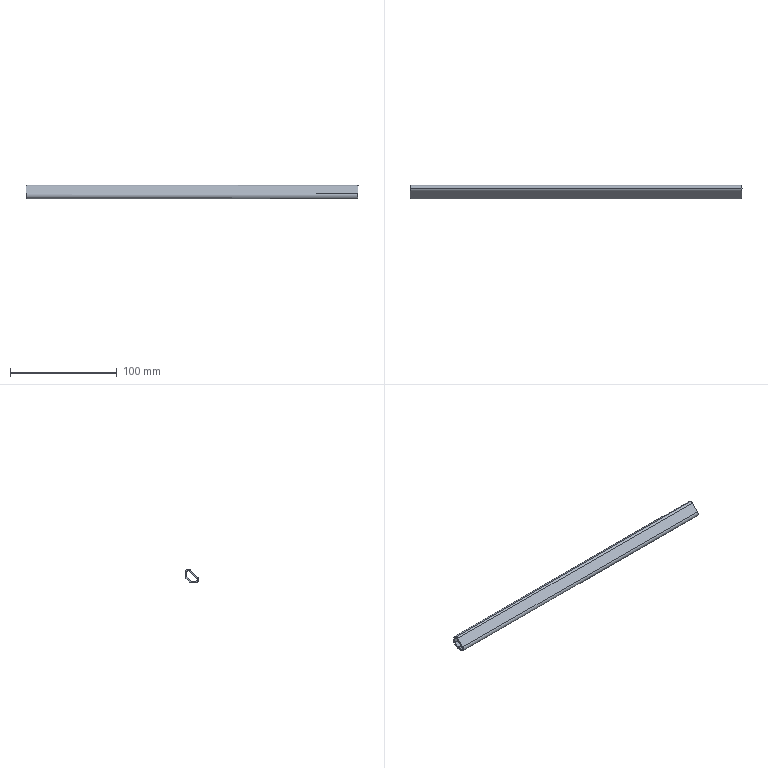Part | SolidWorks | features BaseBody 1 | 1 solid | 20 faces | box 311.635 x 12.741 x 12.993 mm | volume 16541 mm3 | cylinder 10 | plane 10 | commonest cylinder face diameters 3 x3 6 x3 1 x2 4 x2
STEP:
#1=CARTESIAN_POINT('',(151.49,213.806,-273.62));
#2=VERTEX_POINT('',#1);
#3=CARTESIAN_POINT('',(151.488,216.807,-276.619));
#4=VERTEX_POINT('',#3);
#5=CARTESIAN_POINT('',(151.488,213.807,-276.62));
#6=DIRECTION('',(-1.,-0.00003863,0.0008339));
#7=DIRECTION('',(0.0008339,-0.0004454,1.));
#8=AXIS2_PLACEMENT_3D('',#5,#6,#7);
#9=CIRCLE('',#8,3.);
#10=EDGE_CURVE('',#2,#4,#9,.T.);
#11=ORIENTED_EDGE('',*,*,#10,.T.);
#12=CARTESIAN_POINT('',(-160.136,216.795,-276.359));
#13=VERTEX_POINT('',#12);
#14=CARTESIAN_POINT('',(-160.136,216.795,-276.359));
#15=DIRECTION('',(1.,0.00003863,-0.0008339));
#16=VECTOR('',#15,1000.);
#17=LINE('',#14,#16);
#18=EDGE_CURVE('',#13,#4,#17,.T.);
#19=ORIENTED_EDGE('',*,*,#18,.F.);
#20=CARTESIAN_POINT('',(-160.134,213.794,-273.36));
#21=VERTEX_POINT('',#20);
#22=CARTESIAN_POINT('',(-160.136,213.795,-276.36));
#23=DIRECTION('',(1.,0.00003863,-0.0008339));
#24=DIRECTION('',(-0.00003826,1.,0.0004455));
#25=AXIS2_PLACEMENT_3D('',#22,#23,#24);
#26=CIRCLE('',#25,3.);
#27=EDGE_CURVE('',#13,#21,#26,.T.);
#28=ORIENTED_EDGE('',*,*,#27,.T.);
#29=CARTESIAN_POINT('',(-160.134,213.794,-273.36));
#30=DIRECTION('',(1.,0.00003863,-0.0008339));
#31=VECTOR('',#30,1000.);
#32=LINE('',#29,#31);
#33=EDGE_CURVE('',#21,#2,#32,.T.);
#34=ORIENTED_EDGE('',*,*,#33,.T.);
#35=EDGE_LOOP('',(#11,#19,#28,#34));
#36=FACE_OUTER_BOUND('',#35,.T.);
#37=CARTESIAN_POINT('',(48.652,213.803,-276.535));
#38=DIRECTION('',(-1.,-0.00003863,0.0008339));
#39=DIRECTION('',(0.0008339,-0.0004454,1.));
#40=AXIS2_PLACEMENT_3D('',#37,#38,#39);
#41=CYLINDRICAL_SURFACE('',#40,3.);
#42=ADVANCED_FACE('',(#36),#41,.T.);
#43=ORIENTED_EDGE('',*,*,#33,.F.);
#44=CARTESIAN_POINT('',(-160.134,211.673,-274.24));
#45=VERTEX_POINT('',#44);
#46=CARTESIAN_POINT('',(-160.136,213.795,-276.36));
#47=DIRECTION('',(1.,0.00003863,-0.0008339));
#48=DIRECTION('',(0.0008339,-0.0004454,1.));
#49=AXIS2_PLACEMENT_3D('',#46,#47,#48);
#50=CIRCLE('',#49,3.);
#51=EDGE_CURVE('',#21,#45,#50,.T.);
#52=ORIENTED_EDGE('',*,*,#51,.T.);
#53=CARTESIAN_POINT('',(151.49,211.685,-274.5));
#54=VERTEX_POINT('',#53);
#55=CARTESIAN_POINT('',(-160.134,211.673,-274.24));
#56=DIRECTION('',(1.,0.00003863,-0.0008339));
#57=VECTOR('',#56,1000.);
#58=LINE('',#55,#57);
#59=EDGE_CURVE('',#45,#54,#58,.T.);
#60=ORIENTED_EDGE('',*,*,#59,.T.);
#61=CARTESIAN_POINT('',(151.488,213.807,-276.62));
#62=DIRECTION('',(-1.,-0.00003863,0.0008339));
#63=DIRECTION('',(0.0006167,-0.7074,0.7068));
#64=AXIS2_PLACEMENT_3D('',#61,#62,#63);
#65=CIRCLE('',#64,3.);
#66=EDGE_CURVE('',#54,#2,#65,.T.);
#67=ORIENTED_EDGE('',*,*,#66,.T.);
#68=EDGE_LOOP('',(#43,#52,#60,#67));
#69=FACE_OUTER_BOUND('',#68,.T.);
#70=CARTESIAN_POINT('',(48.652,213.803,-276.535));
#71=DIRECTION('',(-1.,-0.00003863,0.0008339));
#72=DIRECTION('',(0.0008339,-0.0004454,1.));
#73=AXIS2_PLACEMENT_3D('',#70,#71,#72);
#74=CYLINDRICAL_SURFACE('',#73,3.);
#75=ADVANCED_FACE('',(#69),#74,.T.);
#76=CARTESIAN_POINT('',(151.489,212.746,-275.56));
#77=VERTEX_POINT('',#76);
#78=CARTESIAN_POINT('',(151.484,206.019,-282.293));
#79=VERTEX_POINT('',#78);
#80=CARTESIAN_POINT('',(151.489,212.746,-275.56));
#81=DIRECTION('',(-0.0005626,-0.7068,-0.7074));
#82=VECTOR('',#81,1000.);
#83=LINE('',#80,#82);
#84=EDGE_CURVE('',#77,#79,#83,.T.);
#85=ORIENTED_EDGE('',*,*,#84,.F.);
#86=CARTESIAN_POINT('',(151.489,213.807,-275.12));
#87=VERTEX_POINT('',#86);
#88=CARTESIAN_POINT('',(151.488,213.807,-276.62));
#89=DIRECTION('',(1.,0.00003863,-0.0008339));
#90=DIRECTION('',(0.0008339,-0.0004454,1.));
#91=AXIS2_PLACEMENT_3D('',#88,#89,#90);
#92=CIRCLE('',#91,1.5);
#93=EDGE_CURVE('',#87,#77,#92,.T.);
#94=ORIENTED_EDGE('',*,*,#93,.F.);
#95=CARTESIAN_POINT('',(151.488,215.307,-276.62));
#96=VERTEX_POINT('',#95);
#97=CARTESIAN_POINT('',(151.488,213.807,-276.62));
#98=DIRECTION('',(1.,0.00003863,-0.0008339));
#99=DIRECTION('',(-0.00003826,1.,0.0004455));
#100=AXIS2_PLACEMENT_3D('',#97,#98,#99);
#101=CIRCLE('',#100,1.5);
#102=EDGE_CURVE('',#96,#87,#101,.T.);
#103=ORIENTED_EDGE('',*,*,#102,.F.);
#104=CARTESIAN_POINT('',(151.484,215.309,-280.668));
#105=VERTEX_POINT('',#104);
#106=CARTESIAN_POINT('',(151.488,215.307,-276.62));
#107=DIRECTION('',(-0.0008339,0.0004454,-1.));
#108=VECTOR('',#107,1000.);
#109=LINE('',#106,#108);
#110=EDGE_CURVE('',#96,#105,#109,.T.);
#111=ORIENTED_EDGE('',*,*,#110,.T.);
#112=CARTESIAN_POINT('',(151.484,215.163,-281.021));
#113=VERTEX_POINT('',#112);
#114=CARTESIAN_POINT('',(151.485,214.809,-280.668));
#115=DIRECTION('',(1.,0.00003863,-0.0008339));
#116=DIRECTION('',(-0.0006167,0.7074,-0.7068));
#117=AXIS2_PLACEMENT_3D('',#114,#115,#116);
#118=CIRCLE('',#117,0.5);
#119=EDGE_CURVE('',#113,#105,#118,.T.);
#120=ORIENTED_EDGE('',*,*,#119,.F.);
#121=CARTESIAN_POINT('',(151.481,211.483,-284.705));
#122=VERTEX_POINT('',#121);
#123=CARTESIAN_POINT('',(151.481,211.483,-284.705));
#124=DIRECTION('',(0.0005626,0.7068,0.7074));
#125=VECTOR('',#124,1000.);
#126=LINE('',#123,#125);
#127=EDGE_CURVE('',#122,#113,#126,.T.);
#128=ORIENTED_EDGE('',*,*,#127,.F.);
#129=CARTESIAN_POINT('',(151.481,211.129,-284.852));
#130=VERTEX_POINT('',#129);
#131=CARTESIAN_POINT('',(151.482,211.129,-284.352));
#132=DIRECTION('',(1.,0.00003863,-0.0008339));
#133=DIRECTION('',(-0.0008339,0.0004481,-1.));
#134=AXIS2_PLACEMENT_3D('',#131,#132,#133);
#135=CIRCLE('',#134,0.5);
#136=EDGE_CURVE('',#130,#122,#135,.T.);
#137=ORIENTED_EDGE('',*,*,#136,.F.);
#138=CARTESIAN_POINT('',(151.481,207.081,-284.853));
#139=VERTEX_POINT('',#138);
#140=CARTESIAN_POINT('',(151.481,211.129,-284.852));
#141=DIRECTION('',(0.00003826,-1.,-0.0004455));
#142=VECTOR('',#141,1000.);
#143=LINE('',#140,#142);
#144=EDGE_CURVE('',#130,#139,#143,.T.);
#145=ORIENTED_EDGE('',*,*,#144,.T.);
#146=CARTESIAN_POINT('',(151.483,207.08,-283.353));
#147=DIRECTION('',(1.,0.00003863,-0.0008339));
#148=DIRECTION('',(0.0006167,-0.7074,0.7068));
#149=AXIS2_PLACEMENT_3D('',#146,#147,#148);
#150=CIRCLE('',#149,1.5);
#151=EDGE_CURVE('',#79,#139,#150,.T.);
#152=ORIENTED_EDGE('',*,*,#151,.F.);
#153=EDGE_LOOP('',(#85,#94,#103,#111,#120,#128,#137,#145,#152));
#154=FACE_BOUND('',#153,.T.);
#155=CARTESIAN_POINT('',(151.48,207.082,-286.353));
#156=VERTEX_POINT('',#155);
#157=CARTESIAN_POINT('',(151.484,204.958,-281.233));
#158=VERTEX_POINT('',#157);
#159=CARTESIAN_POINT('',(151.483,207.08,-283.353));
#160=DIRECTION('',(-1.,-0.00003863,0.0008339));
#161=DIRECTION('',(-0.0008339,0.0004117,-1.));
#162=AXIS2_PLACEMENT_3D('',#159,#160,#161);
#163=CIRCLE('',#162,3.);
#164=EDGE_CURVE('',#156,#158,#163,.T.);
#165=ORIENTED_EDGE('',*,*,#164,.F.);
#166=CARTESIAN_POINT('',(151.48,211.13,-286.351));
#167=VERTEX_POINT('',#166);
#168=CARTESIAN_POINT('',(151.48,211.13,-286.351));
#169=DIRECTION('',(0.00003826,-1.,-0.0004455));
#170=VECTOR('',#169,1000.);
#171=LINE('',#168,#170);
#172=EDGE_CURVE('',#167,#156,#171,.T.);
#173=ORIENTED_EDGE('',*,*,#172,.F.);
#174=CARTESIAN_POINT('',(151.48,212.544,-285.765));
#175=VERTEX_POINT('',#174);
#176=CARTESIAN_POINT('',(151.482,211.129,-284.352));
#177=DIRECTION('',(-1.,-0.00003863,0.0008339));
#178=DIRECTION('',(-0.0006167,0.7074,-0.7068));
#179=AXIS2_PLACEMENT_3D('',#176,#177,#178);
#180=CIRCLE('',#179,2.);
#181=EDGE_CURVE('',#175,#167,#180,.T.);
#182=ORIENTED_EDGE('',*,*,#181,.F.);
#183=CARTESIAN_POINT('',(151.483,216.224,-282.082));
#184=VERTEX_POINT('',#183);
#185=CARTESIAN_POINT('',(151.483,216.224,-282.082));
#186=DIRECTION('',(-0.0005626,-0.7068,-0.7074));
#187=VECTOR('',#186,1000.);
#188=LINE('',#185,#187);
#189=EDGE_CURVE('',#184,#175,#188,.T.);
#190=ORIENTED_EDGE('',*,*,#189,.F.);
#191=CARTESIAN_POINT('',(151.484,216.809,-280.667));
#192=VERTEX_POINT('',#191);
#193=CARTESIAN_POINT('',(151.485,214.809,-280.668));
#194=DIRECTION('',(-1.,-0.00003863,0.0008339));
#195=DIRECTION('',(-0.00003826,1.,0.0004457));
#196=AXIS2_PLACEMENT_3D('',#193,#194,#195);
#197=CIRCLE('',#196,2.);
#198=EDGE_CURVE('',#192,#184,#197,.T.);
#199=ORIENTED_EDGE('',*,*,#198,.F.);
#200=CARTESIAN_POINT('',(151.488,216.807,-276.619));
#201=DIRECTION('',(-0.0008339,0.0004454,-1.));
#202=VECTOR('',#201,1000.);
#203=LINE('',#200,#202);
#204=EDGE_CURVE('',#4,#192,#203,.T.);
#205=ORIENTED_EDGE('',*,*,#204,.F.);
#206=ORIENTED_EDGE('',*,*,#10,.F.);
#207=ORIENTED_EDGE('',*,*,#66,.F.);
#208=CARTESIAN_POINT('',(151.484,204.958,-281.233));
#209=DIRECTION('',(0.0005626,0.7068,0.7074));
#210=VECTOR('',#209,1000.);
#211=LINE('',#208,#210);
#212=EDGE_CURVE('',#158,#54,#211,.T.);
#213=ORIENTED_EDGE('',*,*,#212,.F.);
#214=EDGE_LOOP('',(#165,#173,#182,#190,#199,#205,#206,#207,#213));
#215=FACE_OUTER_BOUND('',#214,.T.);
#216=CARTESIAN_POINT('',(151.48,216.812,-286.349));
#217=DIRECTION('',(1.,0.00003863,-0.0008339));
#218=DIRECTION('',(0.,-0.9989,-0.04628));
#219=AXIS2_PLACEMENT_3D('',#216,#217,#218);
#220=PLANE('',#219);
#221=ADVANCED_FACE('',(#154,#215),#220,.T.);
#222=ORIENTED_EDGE('',*,*,#59,.F.);
#223=CARTESIAN_POINT('',(-160.14,204.946,-280.973));
#224=VERTEX_POINT('',#223);
#225=CARTESIAN_POINT('',(-160.134,211.673,-274.24));
#226=DIRECTION('',(-0.0005626,-0.7068,-0.7074));
#227=VECTOR('',#226,1000.);
#228=LINE('',#225,#227);
#229=EDGE_CURVE('',#45,#224,#228,.T.);
#230=ORIENTED_EDGE('',*,*,#229,.T.);
#231=CARTESIAN_POINT('',(151.484,204.958,-281.233));
#232=DIRECTION('',(-1.,-0.00003863,0.0008339));
#233=VECTOR('',#232,1000.);
#234=LINE('',#231,#233);
#235=EDGE_CURVE('',#158,#224,#234,.T.);
#236=ORIENTED_EDGE('',*,*,#235,.F.);
#237=ORIENTED_EDGE('',*,*,#212,.T.);
#238=EDGE_LOOP('',(#222,#230,#236,#237));
#239=FACE_OUTER_BOUND('',#238,.T.);
#240=CARTESIAN_POINT('',(-2.767,208.316,-277.738));
#241=DIRECTION('',(0.0006167,-0.7074,0.7068));
#242=DIRECTION('',(-1.,-0.0008718,0.));
#243=AXIS2_PLACEMENT_3D('',#240,#241,#242);
#244=PLANE('',#243);
#245=ADVANCED_FACE('',(#239),#244,.T.);
#246=CARTESIAN_POINT('',(-160.144,207.07,-286.093));
#247=VERTEX_POINT('',#246);
#248=CARTESIAN_POINT('',(151.48,207.082,-286.353));
#249=DIRECTION('',(-1.,-0.00003848,0.0008339));
#250=VECTOR('',#249,1000.);
#251=LINE('',#248,#250);
#252=EDGE_CURVE('',#156,#247,#251,.T.);
#253=ORIENTED_EDGE('',*,*,#252,.F.);
#254=ORIENTED_EDGE('',*,*,#164,.T.);
#255=ORIENTED_EDGE('',*,*,#235,.T.);
#256=CARTESIAN_POINT('',(-160.142,207.068,-283.093));
#257=DIRECTION('',(1.,0.00003863,-0.0008339));
#258=DIRECTION('',(0.0006167,-0.7074,0.7068));
#259=AXIS2_PLACEMENT_3D('',#256,#257,#258);
#260=CIRCLE('',#259,3.);
#261=EDGE_CURVE('',#224,#247,#260,.T.);
#262=ORIENTED_EDGE('',*,*,#261,.T.);
#263=EDGE_LOOP('',(#253,#254,#255,#262));
#264=FACE_OUTER_BOUND('',#263,.T.);
#265=CARTESIAN_POINT('',(48.647,207.076,-283.268));
#266=DIRECTION('',(-1.,-0.00003863,0.0008339));
#267=DIRECTION('',(0.0008339,-0.0004454,1.));
#268=AXIS2_PLACEMENT_3D('',#265,#266,#267);
#269=CYLINDRICAL_SURFACE('',#268,3.);
#270=ADVANCED_FACE('',(#264),#269,.T.);
#271=CARTESIAN_POINT('',(-160.143,211.471,-284.445));
#272=VERTEX_POINT('',#271);
#273=CARTESIAN_POINT('',(-160.143,211.117,-284.592));
#274=VERTEX_POINT('',#273);
#275=CARTESIAN_POINT('',(-160.143,211.117,-284.092));
#276=DIRECTION('',(-1.,-0.00003863,0.0008339));
#277=DIRECTION('',(-0.0006167,0.7074,-0.7068));
#278=AXIS2_PLACEMENT_3D('',#275,#276,#277);
#279=CIRCLE('',#278,0.5);
#280=EDGE_CURVE('',#272,#274,#279,.T.);
#281=ORIENTED_EDGE('',*,*,#280,.F.);
#282=CARTESIAN_POINT('',(-160.14,215.151,-280.762));
#283=VERTEX_POINT('',#282);
#284=CARTESIAN_POINT('',(-160.14,215.151,-280.762));
#285=DIRECTION('',(-0.0005626,-0.7068,-0.7074));
#286=VECTOR('',#285,1000.);
#287=LINE('',#284,#286);
#288=EDGE_CURVE('',#283,#272,#287,.T.);
#289=ORIENTED_EDGE('',*,*,#288,.F.);
#290=CARTESIAN_POINT('',(-160.14,215.297,-280.408));
#291=VERTEX_POINT('',#290);
#292=CARTESIAN_POINT('',(-160.14,214.797,-280.408));
#293=DIRECTION('',(-1.,-0.00003863,0.0008339));
#294=DIRECTION('',(-0.00003826,1.,0.0004455));
#295=AXIS2_PLACEMENT_3D('',#292,#293,#294);
#296=CIRCLE('',#295,0.5);
#297=EDGE_CURVE('',#291,#283,#296,.T.);
#298=ORIENTED_EDGE('',*,*,#297,.F.);
#299=CARTESIAN_POINT('',(-160.136,215.295,-276.36));
#300=VERTEX_POINT('',#299);
#301=CARTESIAN_POINT('',(-160.14,215.297,-280.408));
#302=DIRECTION('',(0.0008339,-0.0004454,1.));
#303=VECTOR('',#302,1000.);
#304=LINE('',#301,#303);
#305=EDGE_CURVE('',#291,#300,#304,.T.);
#306=ORIENTED_EDGE('',*,*,#305,.T.);
#307=CARTESIAN_POINT('',(-160.135,213.795,-274.86));
#308=VERTEX_POINT('',#307);
#309=CARTESIAN_POINT('',(-160.136,213.795,-276.36));
#310=DIRECTION('',(-1.,-0.00003863,0.0008339));
#311=DIRECTION('',(0.0008339,-0.0004454,1.));
#312=AXIS2_PLACEMENT_3D('',#309,#310,#311);
#313=CIRCLE('',#312,1.5);
#314=EDGE_CURVE('',#308,#300,#313,.T.);
#315=ORIENTED_EDGE('',*,*,#314,.F.);
#316=CARTESIAN_POINT('',(-160.135,212.734,-275.3));
#317=VERTEX_POINT('',#316);
#318=CARTESIAN_POINT('',(-160.136,213.795,-276.36));
#319=DIRECTION('',(-1.,-0.00003863,0.0008339));
#320=DIRECTION('',(0.0006167,-0.7074,0.7068));
#321=AXIS2_PLACEMENT_3D('',#318,#319,#320);
#322=CIRCLE('',#321,1.5);
#323=EDGE_CURVE('',#317,#308,#322,.T.);
#324=ORIENTED_EDGE('',*,*,#323,.F.);
#325=CARTESIAN_POINT('',(-160.141,206.007,-282.033));
#326=VERTEX_POINT('',#325);
#327=CARTESIAN_POINT('',(-160.141,206.007,-282.033));
#328=DIRECTION('',(0.0005626,0.7068,0.7074));
#329=VECTOR('',#328,1000.);
#330=LINE('',#327,#329);
#331=EDGE_CURVE('',#326,#317,#330,.T.);
#332=ORIENTED_EDGE('',*,*,#331,.F.);
#333=CARTESIAN_POINT('',(-160.143,207.069,-284.593));
#334=VERTEX_POINT('',#333);
#335=CARTESIAN_POINT('',(-160.142,207.068,-283.093));
#336=DIRECTION('',(-1.,-0.00003863,0.0008339));
#337=DIRECTION('',(-0.0008339,0.0004453,-1.));
#338=AXIS2_PLACEMENT_3D('',#335,#336,#337);
#339=CIRCLE('',#338,1.5);
#340=EDGE_CURVE('',#334,#326,#339,.T.);
#341=ORIENTED_EDGE('',*,*,#340,.F.);
#342=CARTESIAN_POINT('',(-160.143,207.069,-284.593));
#343=DIRECTION('',(-0.00003826,1.,0.0004455));
#344=VECTOR('',#343,1000.);
#345=LINE('',#342,#344);
#346=EDGE_CURVE('',#334,#274,#345,.T.);
#347=ORIENTED_EDGE('',*,*,#346,.T.);
#348=EDGE_LOOP('',(#281,#289,#298,#306,#315,#324,#332,#341,#347));
#349=FACE_BOUND('',#348,.T.);
#350=ORIENTED_EDGE('',*,*,#261,.F.);
#351=ORIENTED_EDGE('',*,*,#229,.F.);
#352=ORIENTED_EDGE('',*,*,#51,.F.);
#353=ORIENTED_EDGE('',*,*,#27,.F.);
#354=CARTESIAN_POINT('',(-160.14,216.797,-280.407));
#355=VERTEX_POINT('',#354);
#356=CARTESIAN_POINT('',(-160.14,216.797,-280.407));
#357=DIRECTION('',(0.0008339,-0.0004454,1.));
#358=VECTOR('',#357,1000.);
#359=LINE('',#356,#358);
#360=EDGE_CURVE('',#355,#13,#359,.T.);
#361=ORIENTED_EDGE('',*,*,#360,.F.);
#362=CARTESIAN_POINT('',(-160.141,216.212,-281.822));
#363=VERTEX_POINT('',#362);
#364=CARTESIAN_POINT('',(-160.14,214.797,-280.408));
#365=DIRECTION('',(1.,0.00003863,-0.0008339));
#366=DIRECTION('',(-0.0006167,0.7074,-0.7068));
#367=AXIS2_PLACEMENT_3D('',#364,#365,#366);
#368=CIRCLE('',#367,2.);
#369=EDGE_CURVE('',#363,#355,#368,.T.);
#370=ORIENTED_EDGE('',*,*,#369,.F.);
#371=CARTESIAN_POINT('',(-160.144,212.532,-285.505));
#372=VERTEX_POINT('',#371);
#373=CARTESIAN_POINT('',(-160.144,212.532,-285.505));
#374=DIRECTION('',(0.0005626,0.7068,0.7074));
#375=VECTOR('',#374,1000.);
#376=LINE('',#373,#375);
#377=EDGE_CURVE('',#372,#363,#376,.T.);
#378=ORIENTED_EDGE('',*,*,#377,.F.);
#379=CARTESIAN_POINT('',(-160.144,211.118,-286.092));
#380=VERTEX_POINT('',#379);
#381=CARTESIAN_POINT('',(-160.143,211.117,-284.092));
#382=DIRECTION('',(1.,0.00003863,-0.0008339));
#383=DIRECTION('',(-0.0008339,0.0004461,-1.));
#384=AXIS2_PLACEMENT_3D('',#381,#382,#383);
#385=CIRCLE('',#384,2.);
#386=EDGE_CURVE('',#380,#372,#385,.T.);
#387=ORIENTED_EDGE('',*,*,#386,.F.);
#388=CARTESIAN_POINT('',(-160.144,207.07,-286.093));
#389=DIRECTION('',(-0.00003827,1.,0.0004455));
#390=VECTOR('',#389,1000.);
#391=LINE('',#388,#390);
#392=EDGE_CURVE('',#247,#380,#391,.T.);
#393=ORIENTED_EDGE('',*,*,#392,.F.);
#394=EDGE_LOOP('',(#350,#351,#352,#353,#361,#370,#378,#387,#393));
#395=FACE_OUTER_BOUND('',#394,.T.);
#396=CARTESIAN_POINT('',(-160.145,216.8,-286.089));
#397=DIRECTION('',(-1.,-0.00003863,0.0008339));
#398=DIRECTION('',(-0.00003863,1.,0.));
#399=AXIS2_PLACEMENT_3D('',#396,#397,#398);
#400=PLANE('',#399);
#401=ADVANCED_FACE('',(#349,#395),#400,.T.);
#402=ORIENTED_EDGE('',*,*,#252,.T.);
#403=ORIENTED_EDGE('',*,*,#392,.T.);
#404=CARTESIAN_POINT('',(151.48,211.13,-286.351));
#405=DIRECTION('',(-1.,-0.00003863,0.0008339));
#406=VECTOR('',#405,1000.);
#407=LINE('',#404,#406);
#408=EDGE_CURVE('',#167,#380,#407,.T.);
#409=ORIENTED_EDGE('',*,*,#408,.F.);
#410=ORIENTED_EDGE('',*,*,#172,.T.);
#411=EDGE_LOOP('',(#402,#403,#409,#410));
#412=FACE_OUTER_BOUND('',#411,.T.);
#413=CARTESIAN_POINT('',(-2.774,209.1,-286.224));
#414=DIRECTION('',(-0.0008339,0.0004454,-1.));
#415=DIRECTION('',(-1.,0.,0.0008339));
#416=AXIS2_PLACEMENT_3D('',#413,#414,#415);
#417=PLANE('',#416);
#418=ADVANCED_FACE('',(#412),#417,.T.);
#419=ORIENTED_EDGE('',*,*,#408,.T.);
#420=ORIENTED_EDGE('',*,*,#386,.T.);
#421=CARTESIAN_POINT('',(-160.144,212.532,-285.505));
#422=DIRECTION('',(1.,0.00003863,-0.0008339));
#423=VECTOR('',#422,1000.);
#424=LINE('',#421,#423);
#425=EDGE_CURVE('',#372,#175,#424,.T.);
#426=ORIENTED_EDGE('',*,*,#425,.T.);
#427=ORIENTED_EDGE('',*,*,#181,.T.);
#428=EDGE_LOOP('',(#419,#420,#426,#427));
#429=FACE_OUTER_BOUND('',#428,.T.);
#430=CARTESIAN_POINT('',(48.646,211.125,-284.266));
#431=DIRECTION('',(-1.,-0.00003863,0.0008339));
#432=DIRECTION('',(0.0008339,-0.0004454,1.));
#433=AXIS2_PLACEMENT_3D('',#430,#431,#432);
#434=CYLINDRICAL_SURFACE('',#433,2.);
#435=ADVANCED_FACE('',(#429),#434,.T.);
#436=ORIENTED_EDGE('',*,*,#425,.F.);
#437=ORIENTED_EDGE('',*,*,#377,.T.);
#438=CARTESIAN_POINT('',(151.483,216.224,-282.082));
#439=DIRECTION('',(-1.,-0.00003863,0.0008339));
#440=VECTOR('',#439,1000.);
#441=LINE('',#438,#440);
#442=EDGE_CURVE('',#184,#363,#441,.T.);
#443=ORIENTED_EDGE('',*,*,#442,.F.);
#444=ORIENTED_EDGE('',*,*,#189,.T.);
#445=EDGE_LOOP('',(#436,#437,#443,#444));
#446=FACE_OUTER_BOUND('',#445,.T.);
#447=CARTESIAN_POINT('',(-2.772,214.378,-283.795));
#448=DIRECTION('',(-0.0006167,0.7074,-0.7068));
#449=DIRECTION('',(-1.,0.,0.0008726));
#450=AXIS2_PLACEMENT_3D('',#447,#448,#449);
#451=PLANE('',#450);
#452=ADVANCED_FACE('',(#446),#451,.T.);
#453=CARTESIAN_POINT('',(-160.14,216.797,-280.407));
#454=DIRECTION('',(1.,0.00003863,-0.0008339));
#455=VECTOR('',#454,1000.);
#456=LINE('',#453,#455);
#457=EDGE_CURVE('',#355,#192,#456,.T.);
#458=ORIENTED_EDGE('',*,*,#457,.T.);
#459=ORIENTED_EDGE('',*,*,#198,.T.);
#460=ORIENTED_EDGE('',*,*,#442,.T.);
#461=ORIENTED_EDGE('',*,*,#369,.T.);
#462=EDGE_LOOP('',(#458,#459,#460,#461));
#463=FACE_OUTER_BOUND('',#462,.T.);
#464=CARTESIAN_POINT('',(48.649,214.805,-280.582));
#465=DIRECTION('',(-1.,-0.00003863,0.0008339));
#466=DIRECTION('',(0.0008339,-0.0004454,1.));
#467=AXIS2_PLACEMENT_3D('',#464,#465,#466);
#468=CYLINDRICAL_SURFACE('',#467,2.);
#469=ADVANCED_FACE('',(#463),#468,.T.);
#470=ORIENTED_EDGE('',*,*,#457,.F.);
#471=ORIENTED_EDGE('',*,*,#360,.T.);
#472=ORIENTED_EDGE('',*,*,#18,.T.);
#473=ORIENTED_EDGE('',*,*,#204,.T.);
#474=EDGE_LOOP('',(#470,#471,#472,#473));
#475=FACE_OUTER_BOUND('',#474,.T.);
#476=CARTESIAN_POINT('',(-2.768,216.802,-278.514));
#477=DIRECTION('',(-0.00003826,1.,0.0004455));
#478=DIRECTION('',(0.9963,0.,0.08556));
#479=AXIS2_PLACEMENT_3D('',#476,#477,#478);
#480=PLANE('',#479);
#481=ADVANCED_FACE('',(#475),#480,.T.);
#482=CARTESIAN_POINT('',(-160.143,211.117,-284.592));
#483=DIRECTION('',(1.,0.00003863,-0.0008339));
#484=VECTOR('',#483,1000.);
#485=LINE('',#482,#484);
#486=EDGE_CURVE('',#274,#130,#485,.T.);
#487=ORIENTED_EDGE('',*,*,#486,.F.);
#488=ORIENTED_EDGE('',*,*,#346,.F.);
#489=CARTESIAN_POINT('',(151.481,207.081,-284.853));
#490=DIRECTION('',(-1.,-0.00003863,0.0008339));
#491=VECTOR('',#490,1000.);
#492=LINE('',#489,#491);
#493=EDGE_CURVE('',#139,#334,#492,.T.);
#494=ORIENTED_EDGE('',*,*,#493,.F.);
#495=ORIENTED_EDGE('',*,*,#144,.F.);
#496=EDGE_LOOP('',(#487,#488,#494,#495));
#497=FACE_OUTER_BOUND('',#496,.T.);
#498=CARTESIAN_POINT('',(-2.773,209.099,-284.724));
#499=DIRECTION('',(-0.0008339,0.0004454,-1.));
#500=DIRECTION('',(-1.,0.,0.0008339));
#501=AXIS2_PLACEMENT_3D('',#498,#499,#500);
#502=PLANE('',#501);
#503=ADVANCED_FACE('',(#497),#502,.F.);
#504=CARTESIAN_POINT('',(-160.141,206.007,-282.033));
#505=DIRECTION('',(1.,0.00003863,-0.0008339));
#506=VECTOR('',#505,1000.);
#507=LINE('',#504,#506);
#508=EDGE_CURVE('',#326,#79,#507,.T.);
#509=ORIENTED_EDGE('',*,*,#508,.T.);
#510=ORIENTED_EDGE('',*,*,#151,.T.);
#511=ORIENTED_EDGE('',*,*,#493,.T.);
#512=ORIENTED_EDGE('',*,*,#340,.T.);
#513=EDGE_LOOP('',(#509,#510,#511,#512));
#514=FACE_OUTER_BOUND('',#513,.T.);
#515=CARTESIAN_POINT('',(48.647,207.076,-283.268));
#516=DIRECTION('',(-1.,-0.00003863,0.0008339));
#517=DIRECTION('',(0.0008339,-0.0004454,1.));
#518=AXIS2_PLACEMENT_3D('',#515,#516,#517);
#519=CYLINDRICAL_SURFACE('',#518,1.5);
#520=ADVANCED_FACE('',(#514),#519,.F.);
#521=ORIENTED_EDGE('',*,*,#508,.F.);
#522=ORIENTED_EDGE('',*,*,#331,.T.);
#523=CARTESIAN_POINT('',(151.489,212.746,-275.56));
#524=DIRECTION('',(-1.,-0.00003863,0.0008339));
#525=VECTOR('',#524,1000.);
#526=LINE('',#523,#525);
#527=EDGE_CURVE('',#77,#317,#526,.T.);
#528=ORIENTED_EDGE('',*,*,#527,.F.);
#529=ORIENTED_EDGE('',*,*,#84,.T.);
#530=EDGE_LOOP('',(#521,#522,#528,#529));
#531=FACE_OUTER_BOUND('',#530,.T.);
#532=CARTESIAN_POINT('',(-2.768,209.377,-278.798));
#533=DIRECTION('',(0.0006167,-0.7074,0.7068));
#534=DIRECTION('',(-1.,-0.0008718,0.));
#535=AXIS2_PLACEMENT_3D('',#532,#533,#534);
#536=PLANE('',#535);
#537=ADVANCED_FACE('',(#531),#536,.F.);
#538=ORIENTED_EDGE('',*,*,#93,.T.);
#539=ORIENTED_EDGE('',*,*,#527,.T.);
#540=ORIENTED_EDGE('',*,*,#323,.T.);
#541=CARTESIAN_POINT('',(-160.135,213.795,-274.86));
#542=DIRECTION('',(1.,0.00003863,-0.0008339));
#543=VECTOR('',#542,1000.);
#544=LINE('',#541,#543);
#545=EDGE_CURVE('',#308,#87,#544,.T.);
#546=ORIENTED_EDGE('',*,*,#545,.T.);
#547=EDGE_LOOP('',(#538,#539,#540,#546));
#548=FACE_OUTER_BOUND('',#547,.T.);
#549=CARTESIAN_POINT('',(48.652,213.803,-276.535));
#550=DIRECTION('',(-1.,-0.00003863,0.0008339));
#551=DIRECTION('',(0.0008339,-0.0004454,1.));
#552=AXIS2_PLACEMENT_3D('',#549,#550,#551);
#553=CYLINDRICAL_SURFACE('',#552,1.5);
#554=ADVANCED_FACE('',(#548),#553,.F.);
#555=ORIENTED_EDGE('',*,*,#545,.F.);
#556=ORIENTED_EDGE('',*,*,#314,.T.);
#557=CARTESIAN_POINT('',(-160.136,215.295,-276.36));
#558=DIRECTION('',(1.,0.00003863,-0.0008339));
#559=VECTOR('',#558,1000.);
#560=LINE('',#557,#559);
#561=EDGE_CURVE('',#300,#96,#560,.T.);
#562=ORIENTED_EDGE('',*,*,#561,.T.);
#563=ORIENTED_EDGE('',*,*,#102,.T.);
#564=EDGE_LOOP('',(#555,#556,#562,#563));
#565=FACE_OUTER_BOUND('',#564,.T.);
#566=CARTESIAN_POINT('',(48.652,213.803,-276.535));
#567=DIRECTION('',(-1.,-0.00003863,0.0008339));
#568=DIRECTION('',(0.0008339,-0.0004454,1.));
#569=AXIS2_PLACEMENT_3D('',#566,#567,#568);
#570=CYLINDRICAL_SURFACE('',#569,1.5);
#571=ADVANCED_FACE('',(#565),#570,.F.);
#572=ORIENTED_EDGE('',*,*,#561,.F.);
#573=ORIENTED_EDGE('',*,*,#305,.F.);
#574=CARTESIAN_POINT('',(151.484,215.309,-280.668));
#575=DIRECTION('',(-1.,-0.00003863,0.0008339));
#576=VECTOR('',#575,1000.);
#577=LINE('',#574,#576);
#578=EDGE_CURVE('',#105,#291,#577,.T.);
#579=ORIENTED_EDGE('',*,*,#578,.F.);
#580=ORIENTED_EDGE('',*,*,#110,.F.);
#581=EDGE_LOOP('',(#572,#573,#579,#580));
#582=FACE_OUTER_BOUND('',#581,.T.);
#583=CARTESIAN_POINT('',(-2.768,215.302,-278.515));
#584=DIRECTION('',(-0.00003826,1.,0.0004455));
#585=DIRECTION('',(0.9963,0.,0.08556));
#586=AXIS2_PLACEMENT_3D('',#583,#584,#585);
#587=PLANE('',#586);
#588=ADVANCED_FACE('',(#582),#587,.F.);
#589=CARTESIAN_POINT('',(-160.14,215.151,-280.762));
#590=DIRECTION('',(1.,0.00003863,-0.0008339));
#591=VECTOR('',#590,1000.);
#592=LINE('',#589,#591);
#593=EDGE_CURVE('',#283,#113,#592,.T.);
#594=ORIENTED_EDGE('',*,*,#593,.T.);
#595=ORIENTED_EDGE('',*,*,#119,.T.);
#596=ORIENTED_EDGE('',*,*,#578,.T.);
#597=ORIENTED_EDGE('',*,*,#297,.T.);
#598=EDGE_LOOP('',(#594,#595,#596,#597));
#599=FACE_OUTER_BOUND('',#598,.T.);
#600=CARTESIAN_POINT('',(48.649,214.805,-280.582));
#601=DIRECTION('',(-1.,-0.00003863,0.0008339));
#602=DIRECTION('',(0.0008339,-0.0004454,1.));
#603=AXIS2_PLACEMENT_3D('',#600,#601,#602);
#604=CYLINDRICAL_SURFACE('',#603,0.5);
#605=ADVANCED_FACE('',(#599),#604,.F.);
#606=ORIENTED_EDGE('',*,*,#593,.F.);
#607=ORIENTED_EDGE('',*,*,#288,.T.);
#608=CARTESIAN_POINT('',(151.481,211.483,-284.705));
#609=DIRECTION('',(-1.,-0.00003863,0.0008339));
#610=VECTOR('',#609,1000.);
#611=LINE('',#608,#610);
#612=EDGE_CURVE('',#122,#272,#611,.T.);
#613=ORIENTED_EDGE('',*,*,#612,.F.);
#614=ORIENTED_EDGE('',*,*,#127,.T.);
#615=EDGE_LOOP('',(#606,#607,#613,#614));
#616=FACE_OUTER_BOUND('',#615,.T.);
#617=CARTESIAN_POINT('',(-2.771,213.317,-282.735));
#618=DIRECTION('',(-0.0006167,0.7074,-0.7068));
#619=DIRECTION('',(-1.,0.,0.0008726));
#620=AXIS2_PLACEMENT_3D('',#617,#618,#619);
#621=PLANE('',#620);
#622=ADVANCED_FACE('',(#616),#621,.F.);
#623=ORIENTED_EDGE('',*,*,#612,.T.);
#624=ORIENTED_EDGE('',*,*,#280,.T.);
#625=ORIENTED_EDGE('',*,*,#486,.T.);
#626=ORIENTED_EDGE('',*,*,#136,.T.);
#627=EDGE_LOOP('',(#623,#624,#625,#626));
#628=FACE_OUTER_BOUND('',#627,.T.);
#629=CARTESIAN_POINT('',(48.646,211.125,-284.266));
#630=DIRECTION('',(-1.,-0.00003863,0.0008339));
#631=DIRECTION('',(0.0008339,-0.0004454,1.));
#632=AXIS2_PLACEMENT_3D('',#629,#630,#631);
#633=CYLINDRICAL_SURFACE('',#632,0.5);
#634=ADVANCED_FACE('',(#628),#633,.F.);
#635=CLOSED_SHELL('',(#42,#75,#221,#245,#270,#401,#418,#435,#452,#469,#481,#503,#520,#537,#554,#571,#588,#605,#622,#634));
#636=MANIFOLD_SOLID_BREP('',#635);
#637=CARTESIAN_POINT('',(0.,0.,0.));
#638=DIRECTION('',(0.,0.,1.));
#639=DIRECTION('',(1.,0.,0.));
#640=AXIS2_PLACEMENT_3D('',#637,#638,#639);
#641=(LENGTH_UNIT()NAMED_UNIT(*)SI_UNIT(.MILLI.,.METRE.));
#642=UNCERTAINTY_MEASURE_WITH_UNIT(LENGTH_MEASURE(0.00001),#641,'','');
#643=(NAMED_UNIT(*)PLANE_ANGLE_UNIT()SI_UNIT($,.RADIAN.));
#644=(NAMED_UNIT(*)SI_UNIT($,.STERADIAN.)SOLID_ANGLE_UNIT());
#645=(GEOMETRIC_REPRESENTATION_CONTEXT(3)GLOBAL_UNCERTAINTY_ASSIGNED_CONTEXT((#642))GLOBAL_UNIT_ASSIGNED_CONTEXT((#641,#643,#644))REPRESENTATION_CONTEXT('',''));
#646=ADVANCED_BREP_SHAPE_REPRESENTATION('',(#636,#640),#645);